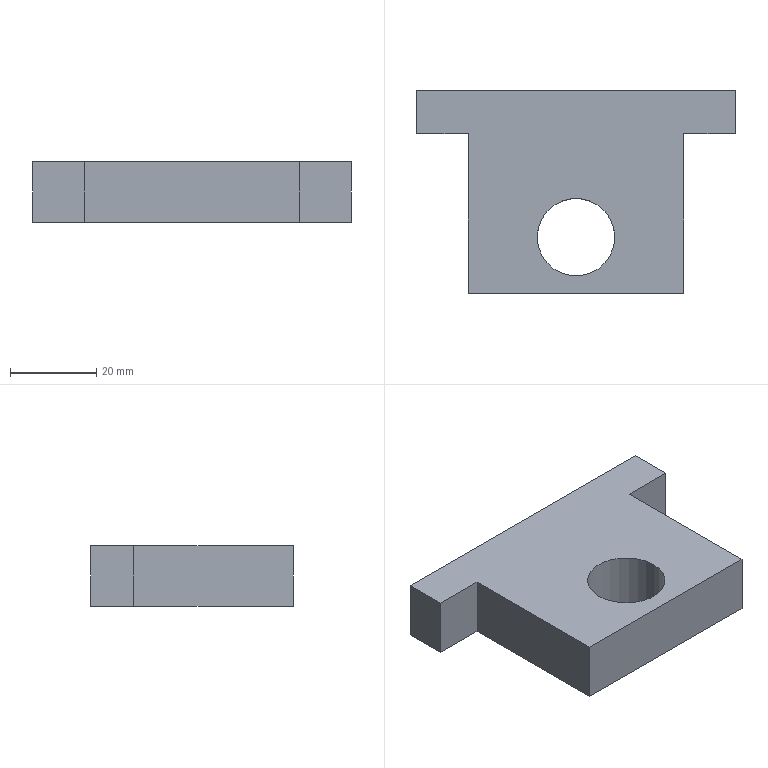Part | SolidWorks | features ICE 2, Extrusion 1 | 1 solid | 12 faces | box 74 x 47 x 14 mm | volume 32697 mm3 | plane 10 | cylinder 2 | commonest cylinder face diameters 18 x2
STEP:
#1=CARTESIAN_POINT('',(-9.,-10.5,7.));
#2=VERTEX_POINT('',#1);
#3=CARTESIAN_POINT('',(9.,-10.5,7.));
#4=VERTEX_POINT('',#3);
#5=CARTESIAN_POINT('',(0.,-10.5,7.));
#6=DIRECTION('',(0.,0.,1.));
#7=DIRECTION('',(-1.,0.,0.));
#8=AXIS2_PLACEMENT_3D('',#5,#6,#7);
#9=CIRCLE('',#8,9.);
#10=EDGE_CURVE('',#2,#4,#9,.T.);
#11=ORIENTED_EDGE('',*,*,#10,.T.);
#12=CARTESIAN_POINT('',(9.,-10.5,-7.));
#13=VERTEX_POINT('',#12);
#14=CARTESIAN_POINT('',(9.,-10.5,7.001));
#15=DIRECTION('',(0.,0.,-1.));
#16=VECTOR('',#15,1000.);
#17=LINE('',#14,#16);
#18=EDGE_CURVE('',#4,#13,#17,.T.);
#19=ORIENTED_EDGE('',*,*,#18,.T.);
#20=CARTESIAN_POINT('',(-9.,-10.5,-7.));
#21=VERTEX_POINT('',#20);
#22=CARTESIAN_POINT('',(0.,-10.5,-7.));
#23=DIRECTION('',(0.,0.,-1.));
#24=DIRECTION('',(-1.,0.,0.));
#25=AXIS2_PLACEMENT_3D('',#22,#23,#24);
#26=CIRCLE('',#25,9.);
#27=EDGE_CURVE('',#13,#21,#26,.T.);
#28=ORIENTED_EDGE('',*,*,#27,.T.);
#29=CARTESIAN_POINT('',(-9.,-10.5,7.001));
#30=DIRECTION('',(0.,0.,-1.));
#31=VECTOR('',#30,1000.);
#32=LINE('',#29,#31);
#33=EDGE_CURVE('',#2,#21,#32,.T.);
#34=ORIENTED_EDGE('',*,*,#33,.F.);
#35=EDGE_LOOP('',(#11,#19,#28,#34));
#36=FACE_OUTER_BOUND('',#35,.T.);
#37=CARTESIAN_POINT('',(0.,-10.5,7.001));
#38=DIRECTION('',(0.,0.,-1.));
#39=DIRECTION('',(-1.,0.,0.));
#40=AXIS2_PLACEMENT_3D('',#37,#38,#39);
#41=CYLINDRICAL_SURFACE('',#40,9.);
#42=ADVANCED_FACE('',(#36),#41,.F.);
#43=CARTESIAN_POINT('',(25.,-23.5,-7.));
#44=VERTEX_POINT('',#43);
#45=CARTESIAN_POINT('',(25.,13.5,-7.));
#46=VERTEX_POINT('',#45);
#47=CARTESIAN_POINT('',(25.,-23.5,-7.));
#48=DIRECTION('',(0.,1.,0.));
#49=VECTOR('',#48,1000.);
#50=LINE('',#47,#49);
#51=EDGE_CURVE('',#44,#46,#50,.T.);
#52=ORIENTED_EDGE('',*,*,#51,.T.);
#53=CARTESIAN_POINT('',(25.,13.5,7.));
#54=VERTEX_POINT('',#53);
#55=CARTESIAN_POINT('',(25.,13.5,-7.));
#56=DIRECTION('',(0.,0.,1.));
#57=VECTOR('',#56,1000.);
#58=LINE('',#55,#57);
#59=EDGE_CURVE('',#46,#54,#58,.T.);
#60=ORIENTED_EDGE('',*,*,#59,.T.);
#61=CARTESIAN_POINT('',(25.,-23.5,7.));
#62=VERTEX_POINT('',#61);
#63=CARTESIAN_POINT('',(25.,-23.5,7.));
#64=DIRECTION('',(0.,1.,0.));
#65=VECTOR('',#64,1000.);
#66=LINE('',#63,#65);
#67=EDGE_CURVE('',#62,#54,#66,.T.);
#68=ORIENTED_EDGE('',*,*,#67,.F.);
#69=CARTESIAN_POINT('',(25.,-23.5,7.));
#70=DIRECTION('',(0.,0.,-1.));
#71=VECTOR('',#70,1000.);
#72=LINE('',#69,#71);
#73=EDGE_CURVE('',#62,#44,#72,.T.);
#74=ORIENTED_EDGE('',*,*,#73,.T.);
#75=EDGE_LOOP('',(#52,#60,#68,#74));
#76=FACE_OUTER_BOUND('',#75,.T.);
#77=CARTESIAN_POINT('',(25.,-23.5,7.));
#78=DIRECTION('',(-1.,0.,0.));
#79=DIRECTION('',(0.,0.,1.));
#80=AXIS2_PLACEMENT_3D('',#77,#78,#79);
#81=PLANE('',#80);
#82=ADVANCED_FACE('',(#76),#81,.F.);
#83=CARTESIAN_POINT('',(37.,23.5,-7.));
#84=VERTEX_POINT('',#83);
#85=CARTESIAN_POINT('',(-37.,23.5,-7.));
#86=VERTEX_POINT('',#85);
#87=CARTESIAN_POINT('',(-25.,23.5,-7.));
#88=DIRECTION('',(-1.,0.,0.));
#89=VECTOR('',#88,1000.);
#90=LINE('',#87,#89);
#91=EDGE_CURVE('',#84,#86,#90,.T.);
#92=ORIENTED_EDGE('',*,*,#91,.T.);
#93=CARTESIAN_POINT('',(-37.,23.5,7.));
#94=VERTEX_POINT('',#93);
#95=CARTESIAN_POINT('',(-37.,23.5,-7.));
#96=DIRECTION('',(0.,0.,1.));
#97=VECTOR('',#96,1000.);
#98=LINE('',#95,#97);
#99=EDGE_CURVE('',#86,#94,#98,.T.);
#100=ORIENTED_EDGE('',*,*,#99,.T.);
#101=CARTESIAN_POINT('',(37.,23.5,7.));
#102=VERTEX_POINT('',#101);
#103=CARTESIAN_POINT('',(-25.,23.5,7.));
#104=DIRECTION('',(-1.,0.,0.));
#105=VECTOR('',#104,1000.);
#106=LINE('',#103,#105);
#107=EDGE_CURVE('',#102,#94,#106,.T.);
#108=ORIENTED_EDGE('',*,*,#107,.F.);
#109=CARTESIAN_POINT('',(37.,23.5,-7.));
#110=DIRECTION('',(0.,0.,-1.));
#111=VECTOR('',#110,1000.);
#112=LINE('',#109,#111);
#113=EDGE_CURVE('',#102,#84,#112,.T.);
#114=ORIENTED_EDGE('',*,*,#113,.T.);
#115=EDGE_LOOP('',(#92,#100,#108,#114));
#116=FACE_OUTER_BOUND('',#115,.T.);
#117=CARTESIAN_POINT('',(-25.,23.5,7.));
#118=DIRECTION('',(0.,-1.,0.));
#119=DIRECTION('',(0.,0.,-1.));
#120=AXIS2_PLACEMENT_3D('',#117,#118,#119);
#121=PLANE('',#120);
#122=ADVANCED_FACE('',(#116),#121,.F.);
#123=CARTESIAN_POINT('',(-25.,13.5,7.));
#124=VERTEX_POINT('',#123);
#125=CARTESIAN_POINT('',(-25.,-23.5,7.));
#126=VERTEX_POINT('',#125);
#127=CARTESIAN_POINT('',(-25.,-23.5,7.));
#128=DIRECTION('',(0.,-1.,0.));
#129=VECTOR('',#128,1000.);
#130=LINE('',#127,#129);
#131=EDGE_CURVE('',#124,#126,#130,.T.);
#132=ORIENTED_EDGE('',*,*,#131,.F.);
#133=CARTESIAN_POINT('',(-25.,13.5,-7.));
#134=VERTEX_POINT('',#133);
#135=CARTESIAN_POINT('',(-25.,13.5,-7.));
#136=DIRECTION('',(0.,0.,-1.));
#137=VECTOR('',#136,1000.);
#138=LINE('',#135,#137);
#139=EDGE_CURVE('',#124,#134,#138,.T.);
#140=ORIENTED_EDGE('',*,*,#139,.T.);
#141=CARTESIAN_POINT('',(-25.,-23.5,-7.));
#142=VERTEX_POINT('',#141);
#143=CARTESIAN_POINT('',(-25.,-23.5,-7.));
#144=DIRECTION('',(0.,-1.,0.));
#145=VECTOR('',#144,1000.);
#146=LINE('',#143,#145);
#147=EDGE_CURVE('',#134,#142,#146,.T.);
#148=ORIENTED_EDGE('',*,*,#147,.T.);
#149=CARTESIAN_POINT('',(-25.,-23.5,7.));
#150=DIRECTION('',(0.,0.,-1.));
#151=VECTOR('',#150,1000.);
#152=LINE('',#149,#151);
#153=EDGE_CURVE('',#126,#142,#152,.T.);
#154=ORIENTED_EDGE('',*,*,#153,.F.);
#155=EDGE_LOOP('',(#132,#140,#148,#154));
#156=FACE_OUTER_BOUND('',#155,.T.);
#157=CARTESIAN_POINT('',(-25.,-23.5,7.));
#158=DIRECTION('',(1.,0.,0.));
#159=DIRECTION('',(0.,0.,-1.));
#160=AXIS2_PLACEMENT_3D('',#157,#158,#159);
#161=PLANE('',#160);
#162=ADVANCED_FACE('',(#156),#161,.F.);
#163=CARTESIAN_POINT('',(-25.,-23.5,-7.));
#164=DIRECTION('',(1.,0.,0.));
#165=VECTOR('',#164,1000.);
#166=LINE('',#163,#165);
#167=EDGE_CURVE('',#142,#44,#166,.T.);
#168=ORIENTED_EDGE('',*,*,#167,.T.);
#169=ORIENTED_EDGE('',*,*,#73,.F.);
#170=CARTESIAN_POINT('',(-25.,-23.5,7.));
#171=DIRECTION('',(1.,0.,0.));
#172=VECTOR('',#171,1000.);
#173=LINE('',#170,#172);
#174=EDGE_CURVE('',#126,#62,#173,.T.);
#175=ORIENTED_EDGE('',*,*,#174,.F.);
#176=ORIENTED_EDGE('',*,*,#153,.T.);
#177=EDGE_LOOP('',(#168,#169,#175,#176));
#178=FACE_OUTER_BOUND('',#177,.T.);
#179=CARTESIAN_POINT('',(-25.,-23.5,7.));
#180=DIRECTION('',(0.,1.,0.));
#181=DIRECTION('',(0.,0.,1.));
#182=AXIS2_PLACEMENT_3D('',#179,#180,#181);
#183=PLANE('',#182);
#184=ADVANCED_FACE('',(#178),#183,.F.);
#185=ORIENTED_EDGE('',*,*,#10,.F.);
#186=CARTESIAN_POINT('',(0.,-10.5,7.));
#187=DIRECTION('',(0.,0.,1.));
#188=DIRECTION('',(-1.,0.,0.));
#189=AXIS2_PLACEMENT_3D('',#186,#187,#188);
#190=CIRCLE('',#189,9.);
#191=EDGE_CURVE('',#4,#2,#190,.T.);
#192=ORIENTED_EDGE('',*,*,#191,.F.);
#193=EDGE_LOOP('',(#185,#192));
#194=FACE_BOUND('',#193,.T.);
#195=ORIENTED_EDGE('',*,*,#67,.T.);
#196=CARTESIAN_POINT('',(37.,13.5,7.));
#197=VERTEX_POINT('',#196);
#198=CARTESIAN_POINT('',(25.,13.5,7.));
#199=DIRECTION('',(1.,0.,0.));
#200=VECTOR('',#199,1000.);
#201=LINE('',#198,#200);
#202=EDGE_CURVE('',#54,#197,#201,.T.);
#203=ORIENTED_EDGE('',*,*,#202,.T.);
#204=CARTESIAN_POINT('',(37.,13.5,7.));
#205=DIRECTION('',(0.,1.,0.));
#206=VECTOR('',#205,1000.);
#207=LINE('',#204,#206);
#208=EDGE_CURVE('',#197,#102,#207,.T.);
#209=ORIENTED_EDGE('',*,*,#208,.T.);
#210=ORIENTED_EDGE('',*,*,#107,.T.);
#211=CARTESIAN_POINT('',(-37.,13.5,7.));
#212=VERTEX_POINT('',#211);
#213=CARTESIAN_POINT('',(-37.,13.5,7.));
#214=DIRECTION('',(0.,1.,0.));
#215=VECTOR('',#214,1000.);
#216=LINE('',#213,#215);
#217=EDGE_CURVE('',#212,#94,#216,.T.);
#218=ORIENTED_EDGE('',*,*,#217,.F.);
#219=CARTESIAN_POINT('',(-25.,13.5,7.));
#220=DIRECTION('',(1.,0.,0.));
#221=VECTOR('',#220,1000.);
#222=LINE('',#219,#221);
#223=EDGE_CURVE('',#212,#124,#222,.T.);
#224=ORIENTED_EDGE('',*,*,#223,.T.);
#225=ORIENTED_EDGE('',*,*,#131,.T.);
#226=ORIENTED_EDGE('',*,*,#174,.T.);
#227=EDGE_LOOP('',(#195,#203,#209,#210,#218,#224,#225,#226));
#228=FACE_OUTER_BOUND('',#227,.T.);
#229=CARTESIAN_POINT('',(0.,0.,7.));
#230=DIRECTION('',(0.,0.,-1.));
#231=DIRECTION('',(-1.,0.,0.));
#232=AXIS2_PLACEMENT_3D('',#229,#230,#231);
#233=PLANE('',#232);
#234=ADVANCED_FACE('',(#194,#228),#233,.F.);
#235=CARTESIAN_POINT('',(0.,-10.5,-7.));
#236=DIRECTION('',(0.,0.,-1.));
#237=DIRECTION('',(-1.,0.,0.));
#238=AXIS2_PLACEMENT_3D('',#235,#236,#237);
#239=CIRCLE('',#238,9.);
#240=EDGE_CURVE('',#21,#13,#239,.T.);
#241=ORIENTED_EDGE('',*,*,#240,.F.);
#242=ORIENTED_EDGE('',*,*,#27,.F.);
#243=EDGE_LOOP('',(#241,#242));
#244=FACE_BOUND('',#243,.T.);
#245=ORIENTED_EDGE('',*,*,#51,.F.);
#246=ORIENTED_EDGE('',*,*,#167,.F.);
#247=ORIENTED_EDGE('',*,*,#147,.F.);
#248=CARTESIAN_POINT('',(-37.,13.5,-7.));
#249=VERTEX_POINT('',#248);
#250=CARTESIAN_POINT('',(-25.,13.5,-7.));
#251=DIRECTION('',(-1.,0.,0.));
#252=VECTOR('',#251,1000.);
#253=LINE('',#250,#252);
#254=EDGE_CURVE('',#134,#249,#253,.T.);
#255=ORIENTED_EDGE('',*,*,#254,.T.);
#256=CARTESIAN_POINT('',(-37.,13.5,-7.));
#257=DIRECTION('',(0.,1.,0.));
#258=VECTOR('',#257,1000.);
#259=LINE('',#256,#258);
#260=EDGE_CURVE('',#249,#86,#259,.T.);
#261=ORIENTED_EDGE('',*,*,#260,.T.);
#262=ORIENTED_EDGE('',*,*,#91,.F.);
#263=CARTESIAN_POINT('',(37.,13.5,-7.));
#264=VERTEX_POINT('',#263);
#265=CARTESIAN_POINT('',(37.,13.5,-7.));
#266=DIRECTION('',(0.,1.,0.));
#267=VECTOR('',#266,1000.);
#268=LINE('',#265,#267);
#269=EDGE_CURVE('',#264,#84,#268,.T.);
#270=ORIENTED_EDGE('',*,*,#269,.F.);
#271=CARTESIAN_POINT('',(25.,13.5,-7.));
#272=DIRECTION('',(-1.,0.,0.));
#273=VECTOR('',#272,1000.);
#274=LINE('',#271,#273);
#275=EDGE_CURVE('',#264,#46,#274,.T.);
#276=ORIENTED_EDGE('',*,*,#275,.T.);
#277=EDGE_LOOP('',(#245,#246,#247,#255,#261,#262,#270,#276));
#278=FACE_OUTER_BOUND('',#277,.T.);
#279=CARTESIAN_POINT('',(0.,0.,-7.));
#280=DIRECTION('',(0.,0.,-1.));
#281=DIRECTION('',(-1.,0.,0.));
#282=AXIS2_PLACEMENT_3D('',#279,#280,#281);
#283=PLANE('',#282);
#284=ADVANCED_FACE('',(#244,#278),#283,.T.);
#285=ORIENTED_EDGE('',*,*,#18,.F.);
#286=ORIENTED_EDGE('',*,*,#191,.T.);
#287=ORIENTED_EDGE('',*,*,#33,.T.);
#288=ORIENTED_EDGE('',*,*,#240,.T.);
#289=EDGE_LOOP('',(#285,#286,#287,#288));
#290=FACE_OUTER_BOUND('',#289,.T.);
#291=CARTESIAN_POINT('',(0.,-10.5,7.001));
#292=DIRECTION('',(0.,0.,-1.));
#293=DIRECTION('',(-1.,0.,0.));
#294=AXIS2_PLACEMENT_3D('',#291,#292,#293);
#295=CYLINDRICAL_SURFACE('',#294,9.);
#296=ADVANCED_FACE('',(#290),#295,.F.);
#297=ORIENTED_EDGE('',*,*,#113,.F.);
#298=ORIENTED_EDGE('',*,*,#208,.F.);
#299=CARTESIAN_POINT('',(37.,13.5,-7.));
#300=DIRECTION('',(0.,0.,-1.));
#301=VECTOR('',#300,1000.);
#302=LINE('',#299,#301);
#303=EDGE_CURVE('',#197,#264,#302,.T.);
#304=ORIENTED_EDGE('',*,*,#303,.T.);
#305=ORIENTED_EDGE('',*,*,#269,.T.);
#306=EDGE_LOOP('',(#297,#298,#304,#305));
#307=FACE_OUTER_BOUND('',#306,.T.);
#308=CARTESIAN_POINT('',(37.,13.5,-7.));
#309=DIRECTION('',(1.,0.,0.));
#310=DIRECTION('',(0.,0.,-1.));
#311=AXIS2_PLACEMENT_3D('',#308,#309,#310);
#312=PLANE('',#311);
#313=ADVANCED_FACE('',(#307),#312,.T.);
#314=ORIENTED_EDGE('',*,*,#59,.F.);
#315=ORIENTED_EDGE('',*,*,#275,.F.);
#316=ORIENTED_EDGE('',*,*,#303,.F.);
#317=ORIENTED_EDGE('',*,*,#202,.F.);
#318=EDGE_LOOP('',(#314,#315,#316,#317));
#319=FACE_OUTER_BOUND('',#318,.T.);
#320=CARTESIAN_POINT('',(0.,13.5,0.));
#321=DIRECTION('',(0.,1.,0.));
#322=DIRECTION('',(0.,0.,1.));
#323=AXIS2_PLACEMENT_3D('',#320,#321,#322);
#324=PLANE('',#323);
#325=ADVANCED_FACE('',(#319),#324,.F.);
#326=ORIENTED_EDGE('',*,*,#99,.F.);
#327=ORIENTED_EDGE('',*,*,#260,.F.);
#328=CARTESIAN_POINT('',(-37.,13.5,-7.));
#329=DIRECTION('',(0.,0.,1.));
#330=VECTOR('',#329,1000.);
#331=LINE('',#328,#330);
#332=EDGE_CURVE('',#249,#212,#331,.T.);
#333=ORIENTED_EDGE('',*,*,#332,.T.);
#334=ORIENTED_EDGE('',*,*,#217,.T.);
#335=EDGE_LOOP('',(#326,#327,#333,#334));
#336=FACE_OUTER_BOUND('',#335,.T.);
#337=CARTESIAN_POINT('',(-37.,13.5,-7.));
#338=DIRECTION('',(-1.,0.,0.));
#339=DIRECTION('',(0.,0.,1.));
#340=AXIS2_PLACEMENT_3D('',#337,#338,#339);
#341=PLANE('',#340);
#342=ADVANCED_FACE('',(#336),#341,.T.);
#343=ORIENTED_EDGE('',*,*,#139,.F.);
#344=ORIENTED_EDGE('',*,*,#223,.F.);
#345=ORIENTED_EDGE('',*,*,#332,.F.);
#346=ORIENTED_EDGE('',*,*,#254,.F.);
#347=EDGE_LOOP('',(#343,#344,#345,#346));
#348=FACE_OUTER_BOUND('',#347,.T.);
#349=CARTESIAN_POINT('',(0.,13.5,0.));
#350=DIRECTION('',(0.,-1.,0.));
#351=DIRECTION('',(0.,0.,-1.));
#352=AXIS2_PLACEMENT_3D('',#349,#350,#351);
#353=PLANE('',#352);
#354=ADVANCED_FACE('',(#348),#353,.T.);
#355=CLOSED_SHELL('',(#42,#82,#122,#162,#184,#234,#284,#296,#313,#325,#342,#354));
#356=MANIFOLD_SOLID_BREP('',#355);
#357=CARTESIAN_POINT('',(0.,0.,0.));
#358=DIRECTION('',(0.,0.,1.));
#359=DIRECTION('',(1.,0.,0.));
#360=AXIS2_PLACEMENT_3D('',#357,#358,#359);
#361=(LENGTH_UNIT()NAMED_UNIT(*)SI_UNIT(.MILLI.,.METRE.));
#362=UNCERTAINTY_MEASURE_WITH_UNIT(LENGTH_MEASURE(0.00001),#361,'','');
#363=(NAMED_UNIT(*)PLANE_ANGLE_UNIT()SI_UNIT($,.RADIAN.));
#364=(NAMED_UNIT(*)SI_UNIT($,.STERADIAN.)SOLID_ANGLE_UNIT());
#365=(GEOMETRIC_REPRESENTATION_CONTEXT(3)GLOBAL_UNCERTAINTY_ASSIGNED_CONTEXT((#362))GLOBAL_UNIT_ASSIGNED_CONTEXT((#361,#363,#364))REPRESENTATION_CONTEXT('',''));
#366=ADVANCED_BREP_SHAPE_REPRESENTATION('',(#356,#360),#365);